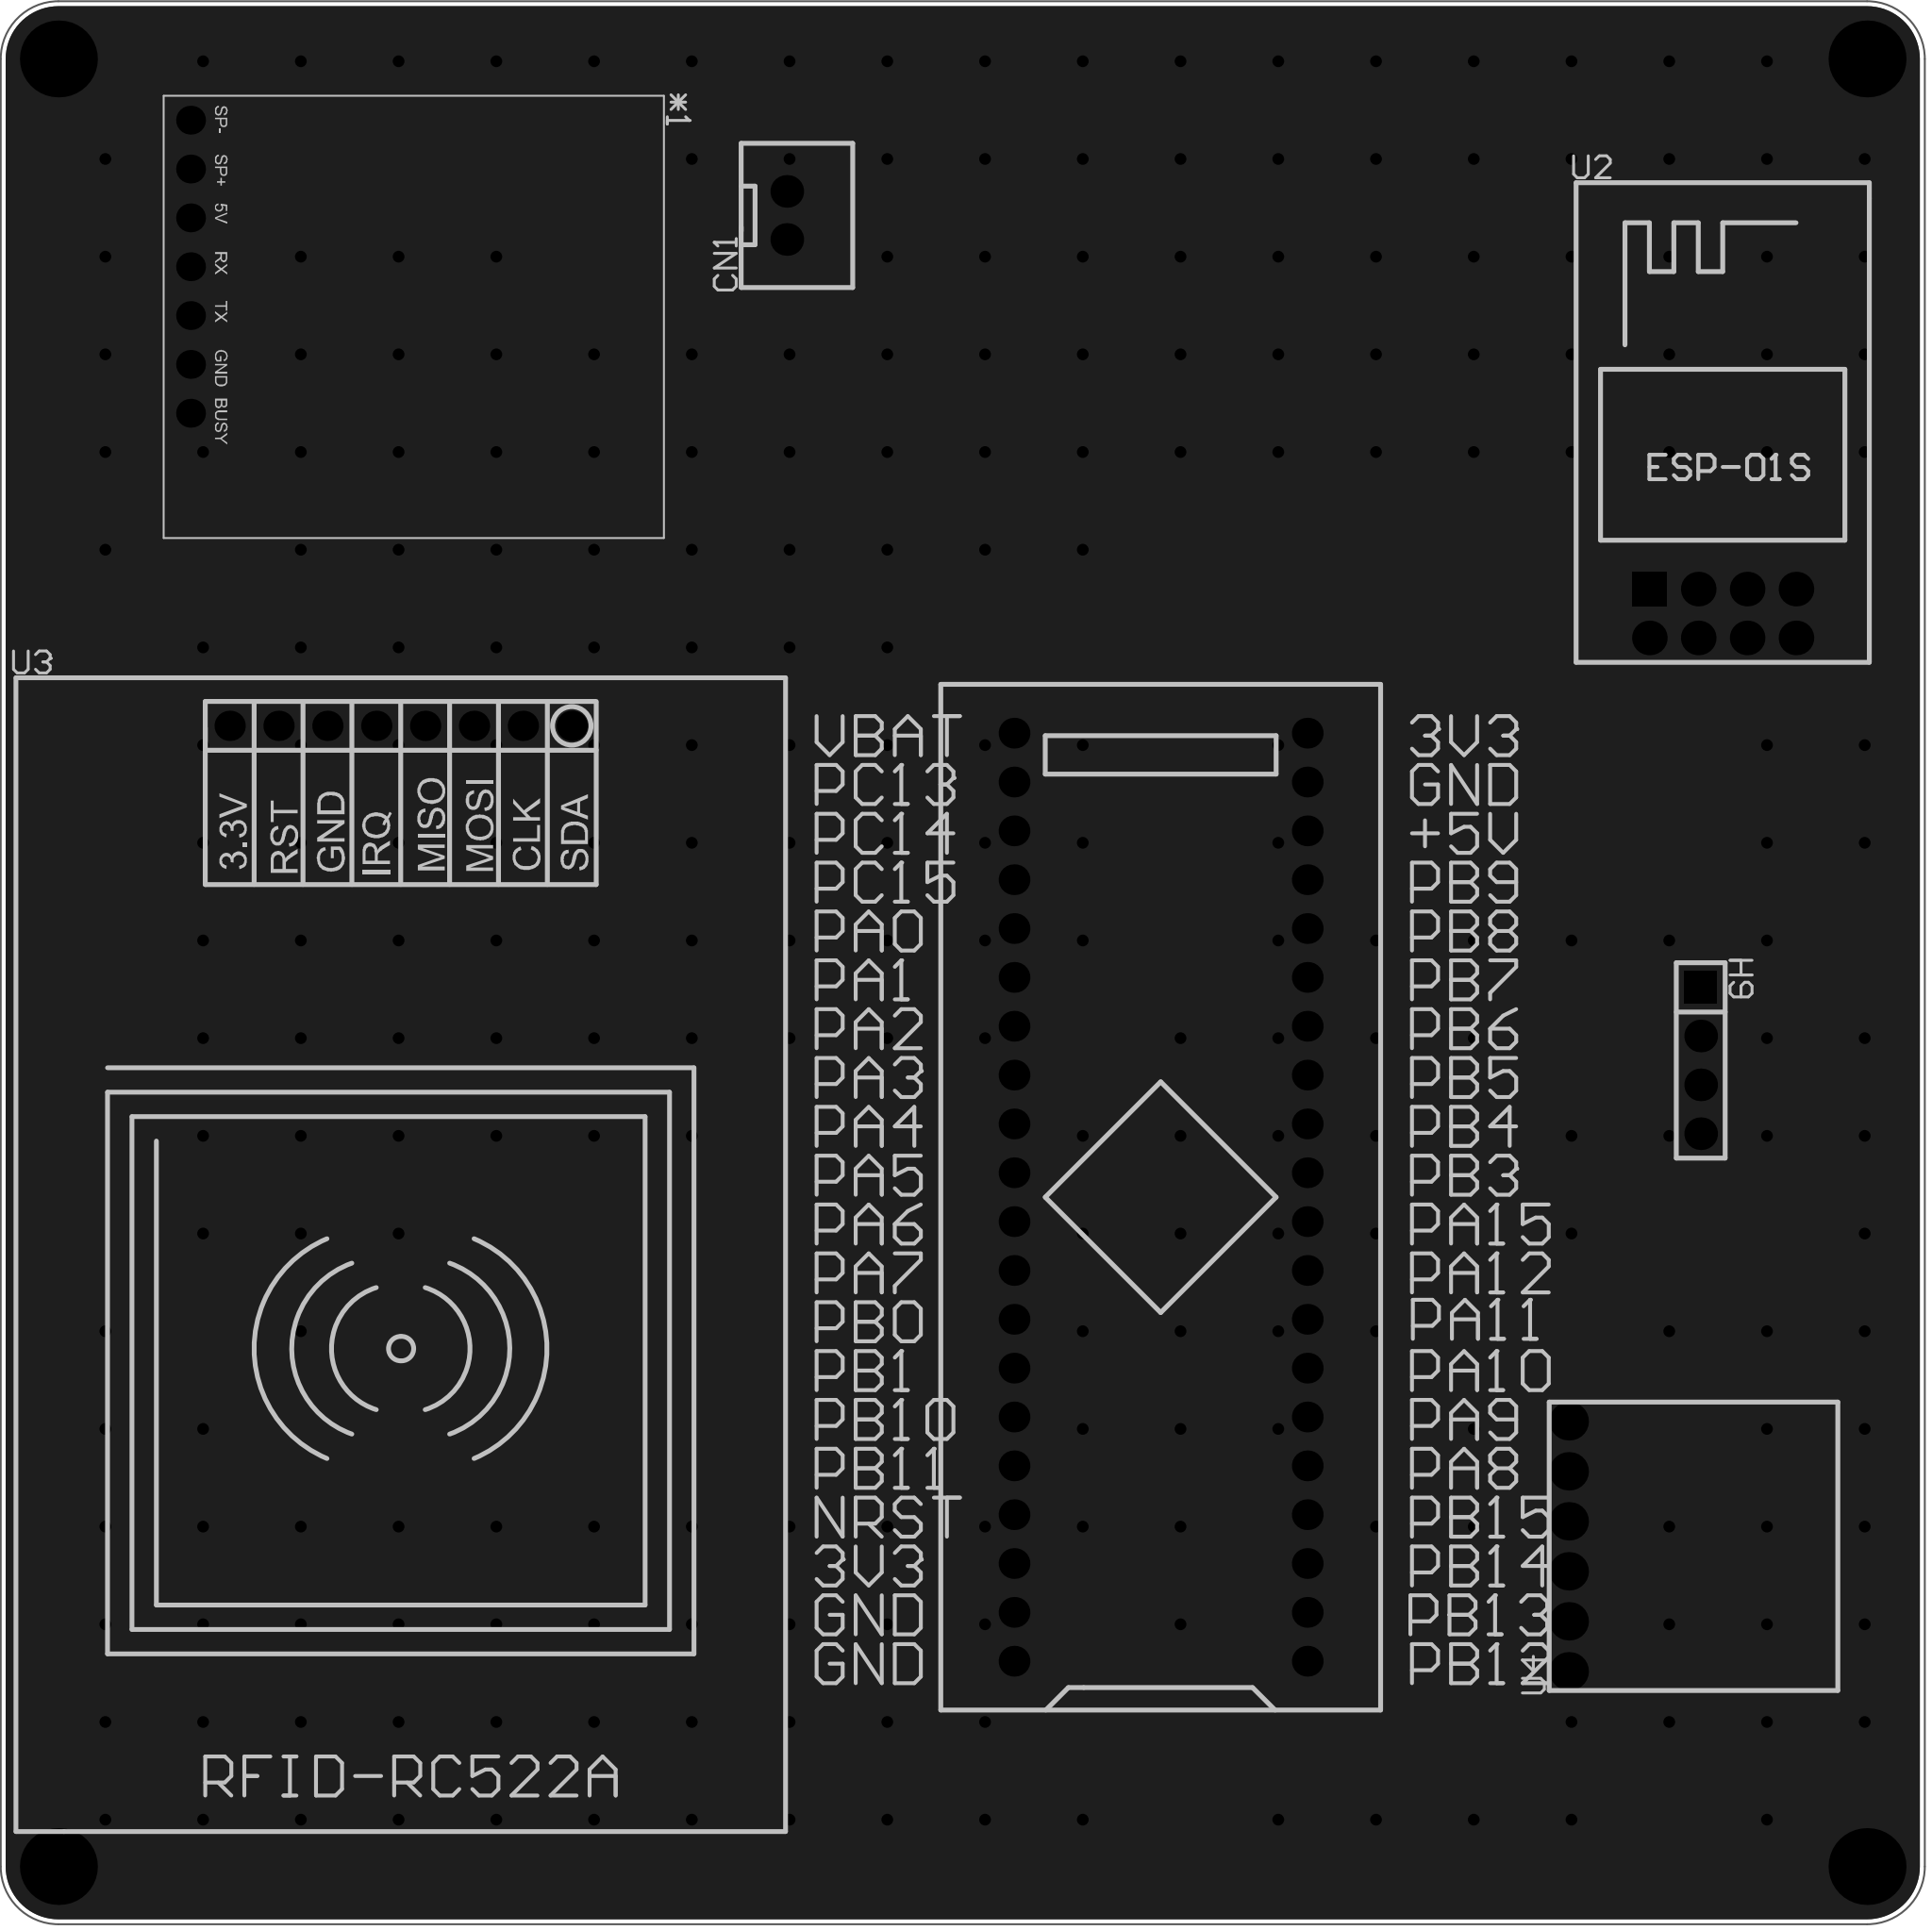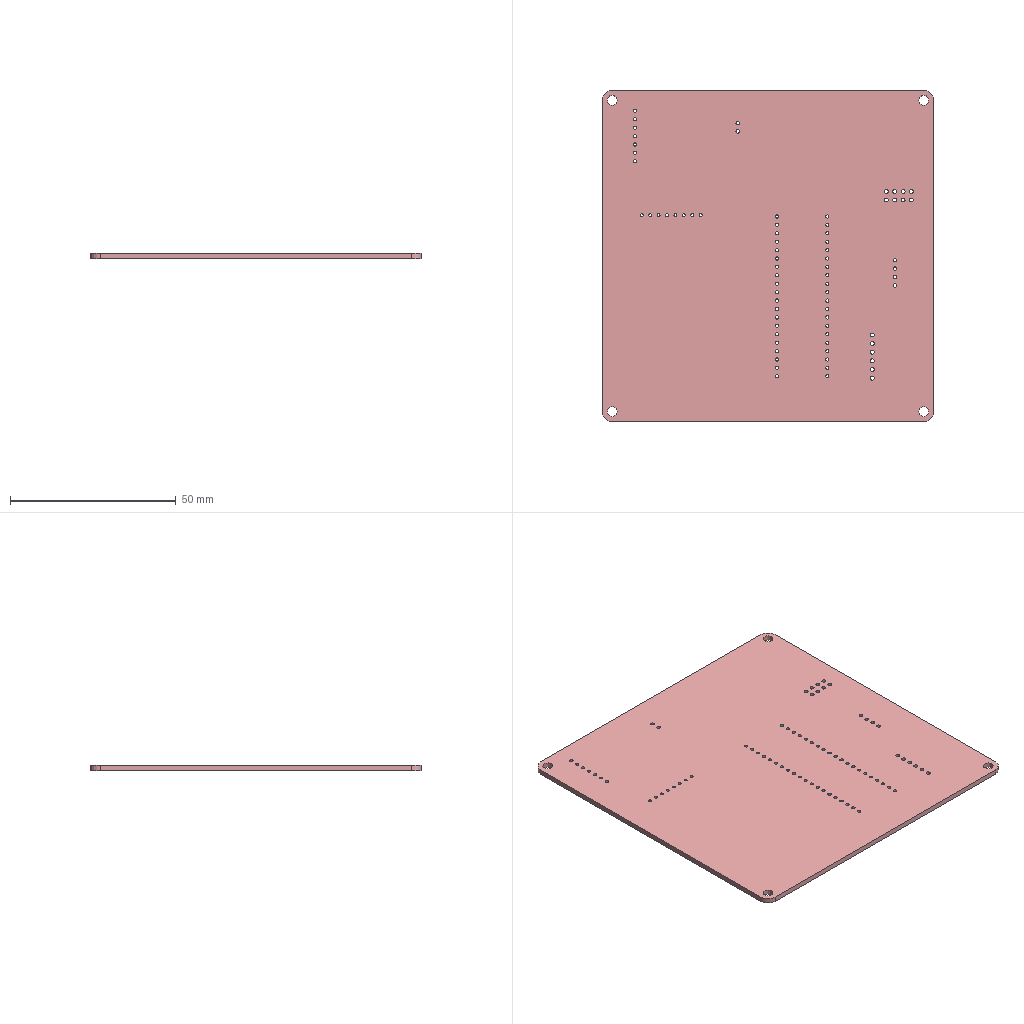Circuit board layout | Altium Designer | box 100 x 100 x 1.6 mm
Layer stack:
# Altium Designer layer stack of  (unit mm; dielectric type: 0 none, 1 core, 2 prepreg, 3 surface material)
index,name,kind,layer,copper_thickness_mm,dielectric_type,dielectric_thickness_mm,dielectric_material,dielectric_constant
0,Top Paste Mask Layer,other,,,,,,
1,Top Silkscreen Layer,other,,,,,,
2,Top Solder Mask Layer,dielectric,,,3,0.01,,3.3
3,Top Layer,copper,Top Layer,0.035,,,,
4,Dielectric1,dielectric,,,3,1.51,FR4,4.5
5,Bottom Layer,copper,Bottom Layer,0.035,,,,
6,Bottom Solder Mask Layer,dielectric,,,3,0.01,,3.3
7,Bottom Silkscreen Layer,other,,,,,,
8,Bottom Paste Mask Layer,other,,,,,,
# drill layer pairs: low layer,high layer
drill_pair,Top Layer,Bottom Layer
Part placement:
Designator,Comment,Layer,Footprint,Center-X(mm),Center-Y(mm),Rotation
U1,STM32F103C8T6-Card,TopLayer,CONN-TH_L53.3-W22.9_STM32F103C8T6-CARD,151.638,118.745,90
*1,LU6288,TopLayer,LU6288,101.219,167.132,270
CN1,XH2.54*2P_直插,TopLayer,CONN-TH_2P-P2.50-XH2.54-2P,132.207,169.799,90
H9,,TopLayer,HDR-TH_4P-P2.54-V-M,179.705,125.857,270
U2,ESP-01S,TopLayer,WIFIM-TH_ESP-01S,180.848,149.098,0
U3,,TopLayer,RC522,112.141,143.256,0
U4,,TopLayer,W25Q64,172.847,100.591,90
Pad and via stacks:
# Altium Designer via and pad stacks of  (unit mm). Each distinct definition once, with the count of objects using it.
# via: kind,start_layer,end_layer,hole_mm,diameter_mm,mode(0 simple;1 top-mid-bottom;2 full stack),diameter_per_layer,count,example_net
# pad: kind,layer,hole_mm,hole_type(0 round;1 square;2 slot),plating,top_size,top_shape(1 round;2 rect;3 octagon;9 rounded rect),mid_size,bottom_size,mode,footprint,size_per_layer,count,example
pad,Multi-Layer,3,0,plated,4x4,1,4x4,4x4,0,,,4,1
pad,Multi-Layer,1,0,plated,1.6x1.6,1,1.6x1.6,1.6x1.6,0,CONN-TH_L53.3-W22.9_STM32F103C8T6-CARD,,40,U1.1
pad,Multi-Layer,1,0,plated,1.5x1.5,1,1.5x1.5,1.5x1.5,0,LU6288,,7,*1.1
pad,Multi-Layer,1.05,0,plated,1.7x1.7,1,1.7x1.7,1.7x1.7,0,CONN-TH_2P-P2.50-XH2.54-2P,,2,CN1.2
pad,Multi-Layer,1.1,0,plated,1.7x1.7,2,1.7x1.7,1.7x1.7,0,HDR-TH_4P-P2.54-V-M,,1,H9.1
pad,Multi-Layer,1.1,0,plated,1.7x1.7,1,1.7x1.7,1.7x1.7,0,HDR-TH_4P-P2.54-V-M,,3,H9.2
pad,Multi-Layer,1.2,0,plated,1.8x1.8,2,1.8x1.8,1.8x1.8,0,WIFIM-TH_ESP-01S,,1,U2.1
pad,Multi-Layer,1.2,0,plated,1.8x1.8,1,1.8x1.8,1.8x1.8,0,WIFIM-TH_ESP-01S,,7,U2.2
pad,Multi-Layer,0.889,0,plated,1.575x1.575,1,1.575x1.575,1.575x1.575,0,RC522,,8,U3.8
pad,Multi-Layer,1.2,0,plated,2x2,1,2x2,2x2,0,W25Q64,,6,U4.1
via,Top Layer,Bottom Layer,0.3048,0.61,0,,259,GND
Copper pours:
name,layer,net,type(0 solid;1 hatched;2 none)
Bottom Layer-GND,Bottom Layer,GND,0
Top Layer-GND,Top Layer,GND,0
Design rules, without the lines most boards share:
# Altium Designer design rules of  (exported by Altium Designer, unit mm)
# columns: name | kind | enabled | priority | scope1 | scope2 | descriptor | typed fields (field=value)
Copper_copperRegion_copperThickness1oz | 0 | disabled | 4 | All | All | Clearance Constraint (Gap=5.984mil) (Disabled)(All),(All) | gap=0.152
Copper_copperRegion_copperThickness1oz_1 | 63 | disabled | 4 | All | All | Board Clearance Constraint (Gap=0mil) (Disabled)(All) |
Copper_copperRegion_Copper_copperRegion | 0 | disabled | 5 | All | All | Clearance Constraint (Gap=5.984mil) (Disabled)(All),(All) | gap=0.152
Copper_copperRegion_Copper_copperRegion_1 | 63 | disabled | 5 | All | All | Board Clearance Constraint (Gap=0mil) (Disabled)(All) |
copperThickness1oz | 0 | enabled | 6 | All | All | Clearance Constraint (Gap=5.984mil) (All),(All) | gap=0.152
copperThickness1oz_1 | 63 | enabled | 6 | All | All | Board Clearance Constraint (Gap=0mil) (All) |
copperRegion_copperThickness1oz | 20 | disabled | 1 | All | All | Polygon Connect Rule(Relief Connect )(Conductor Width=10mil) (Relief Angle=90 Angle) (Entries=4) (Air Gap Width=10mil) (Disabled)(All),(All) | connect_style(0=relief,1=direct,2=none)=0 relief_conductor_width=0.254 relief_entries=4
copperRegion_Copper_copperRegion | 20 | disabled | 2 | All | All | Polygon Connect Rule(Relief Connect )(Conductor Width=10mil) (Relief Angle=90 Angle) (Entries=4) (Air Gap Width=10mil) (Disabled)(All),(All) | connect_style(0=relief,1=direct,2=none)=0 relief_conductor_width=0.254 relief_entries=4
copperRegion | 20 | enabled | 3 | All | All | Polygon Connect Rule(Relief Connect )(Conductor Width=10mil) (Relief Angle=90 Angle) (Entries=4) (Air Gap Width=10mil) (All),(All) | connect_style(0=relief,1=direct,2=none)=0 relief_conductor_width=0.254 relief_entries=4